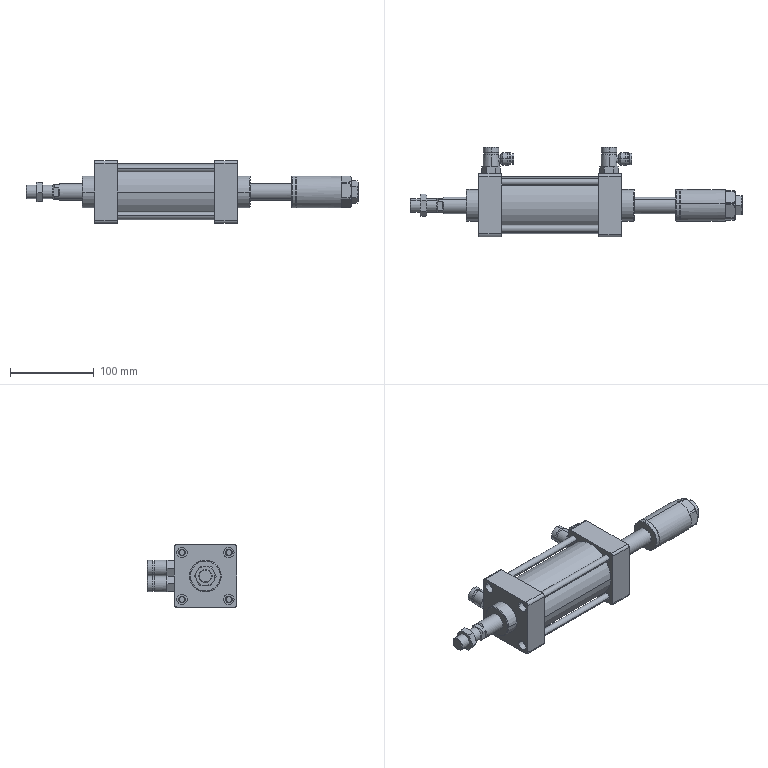Part | SolidWorks | 7 solids | 481 faces | box 397 x 107 x 75 mm | volume 672153 mm3 | plane 163 | cylinder 162 | cone 136 | torus 18 | sphere 2 | commonest cylinder face diameters 6.647 x16 12.5 x16 8 x12 10.1 x8 14.4 x8 20 x8